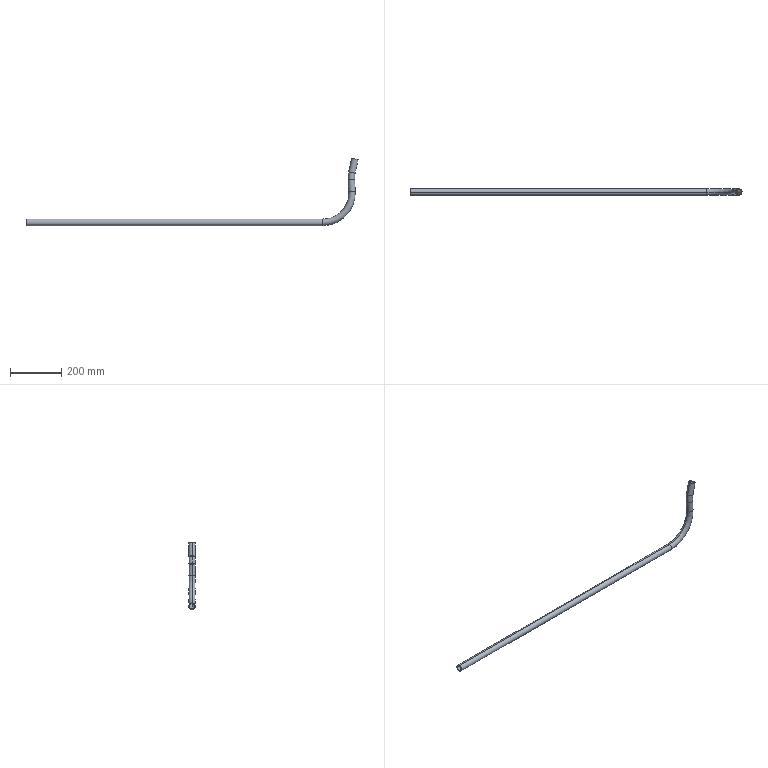Part | STEP file | PN_0018_Default<As Machined> | 1 solid | 26 faces | box 1294 x 25.4 x 262.259 mm | volume 292213 mm3 | cylinder 16 | torus 8 | plane 2 | commonest cylinder face diameters 19.8 x6 25.4 x6 4.2 x4
STEP:
#1=CARTESIAN_POINT('',(312.929,0.,218.744));
#2=VERTEX_POINT('',#1);
#3=CARTESIAN_POINT('',(293.156,0.,217.708));
#4=VERTEX_POINT('',#3);
#5=CARTESIAN_POINT('',(303.043,0.,218.226));
#6=DIRECTION('',(0.05234,0.,-0.9986));
#7=AXIS2_PLACEMENT_3D('',#5,#6,$);
#8=CIRCLE('',#7,9.9);
#9=EDGE_CURVE('',#2,#4,#8,.T.);
#10=ORIENTED_EDGE('',*,*,#9,.T.);
#11=CARTESIAN_POINT('',(295.612,0.,248.912));
#12=VERTEX_POINT('',#11);
#13=CARTESIAN_POINT('',(412.892,0.,223.983));
#14=DIRECTION('',(0.,1.,0.));
#15=AXIS2_PLACEMENT_3D('',#13,#14,$);
#16=CIRCLE('',#15,119.9);
#17=EDGE_CURVE('',#4,#12,#16,.T.);
#18=ORIENTED_EDGE('',*,*,#17,.T.);
#19=CARTESIAN_POINT('',(314.979,0.,244.795));
#20=VERTEX_POINT('',#19);
#21=CARTESIAN_POINT('',(305.296,0.,246.853));
#22=DIRECTION('',(-0.2079,0.,-0.9781));
#23=AXIS2_PLACEMENT_3D('',#21,#22,$);
#24=CIRCLE('',#23,9.9);
#25=EDGE_CURVE('',#20,#12,#24,.T.);
#26=ORIENTED_EDGE('',*,*,#25,.F.);
#27=CARTESIAN_POINT('',(412.892,0.,223.983));
#28=DIRECTION('',(0.,1.,0.));
#29=AXIS2_PLACEMENT_3D('',#27,#28,$);
#30=CIRCLE('',#29,100.1);
#31=EDGE_CURVE('',#2,#20,#30,.T.);
#32=ORIENTED_EDGE('',*,*,#31,.F.);
#33=EDGE_LOOP('',(#10,#18,#26,#32));
#34=FACE_OUTER_BOUND('',#33,.T.);
#35=CARTESIAN_POINT('',(412.892,0.,223.983));
#36=DIRECTION('',(0.,1.,0.));
#37=DIRECTION('',(0.,0.,-1.));
#38=AXIS2_PLACEMENT_3D('',#35,#36,#37);
#39=TOROIDAL_SURFACE('',#38,110.,9.9);
#40=ADVANCED_FACE('',(#34),#39,.F.);
#41=CARTESIAN_POINT('',(315.329,0.,172.946));
#42=VERTEX_POINT('',#41);
#43=CARTESIAN_POINT('',(295.556,0.,171.91));
#44=VERTEX_POINT('',#43);
#45=CARTESIAN_POINT('',(305.443,0.,172.428));
#46=DIRECTION('',(-0.05234,0.,0.9986));
#47=AXIS2_PLACEMENT_3D('',#45,#46,$);
#48=CIRCLE('',#47,9.9);
#49=EDGE_CURVE('',#42,#44,#48,.F.);
#50=ORIENTED_EDGE('',*,*,#49,.T.);
#51=CARTESIAN_POINT('',(295.556,0.,171.91));
#52=DIRECTION('',(-0.05234,0.,0.9986));
#53=VECTOR('',#52,1.);
#54=LINE('',#51,#53);
#55=EDGE_CURVE('',#44,#4,#54,.T.);
#56=ORIENTED_EDGE('',*,*,#55,.T.);
#57=ORIENTED_EDGE('',*,*,#9,.F.);
#58=CARTESIAN_POINT('',(315.329,0.,172.946));
#59=DIRECTION('',(-0.05234,0.,0.9986));
#60=VECTOR('',#59,1.);
#61=LINE('',#58,#60);
#62=EDGE_CURVE('',#42,#2,#61,.T.);
#63=ORIENTED_EDGE('',*,*,#62,.F.);
#64=EDGE_LOOP('',(#50,#56,#57,#63));
#65=FACE_OUTER_BOUND('',#64,.T.);
#66=CARTESIAN_POINT('',(305.443,0.,172.428));
#67=DIRECTION('',(-0.05234,0.,0.9986));
#68=DIRECTION('',(-0.9986,0.,-0.05234));
#69=AXIS2_PLACEMENT_3D('',#66,#67,#68);
#70=CYLINDRICAL_SURFACE('',#69,9.9);
#71=ADVANCED_FACE('',(#65),#70,.F.);
#72=ORIENTED_EDGE('',*,*,#17,.F.);
#73=CARTESIAN_POINT('',(303.043,0.,218.226));
#74=DIRECTION('',(0.05234,0.,-0.9986));
#75=AXIS2_PLACEMENT_3D('',#73,#74,$);
#76=CIRCLE('',#75,9.9);
#77=EDGE_CURVE('',#4,#2,#76,.T.);
#78=ORIENTED_EDGE('',*,*,#77,.T.);
#79=ORIENTED_EDGE('',*,*,#31,.T.);
#80=CARTESIAN_POINT('',(305.296,0.,246.853));
#81=DIRECTION('',(-0.2079,0.,-0.9781));
#82=AXIS2_PLACEMENT_3D('',#80,#81,$);
#83=CIRCLE('',#82,9.9);
#84=EDGE_CURVE('',#12,#20,#83,.T.);
#85=ORIENTED_EDGE('',*,*,#84,.F.);
#86=EDGE_LOOP('',(#72,#78,#79,#85));
#87=FACE_OUTER_BOUND('',#86,.T.);
#88=CARTESIAN_POINT('',(412.892,0.,223.983));
#89=DIRECTION('',(0.,1.,0.));
#90=DIRECTION('',(0.,0.,-1.));
#91=AXIS2_PLACEMENT_3D('',#88,#89,#90);
#92=TOROIDAL_SURFACE('',#91,110.,9.9);
#93=ADVANCED_FACE('',(#87),#92,.F.);
#94=ORIENTED_EDGE('',*,*,#25,.T.);
#95=CARTESIAN_POINT('',(306.777,0.,301.438));
#96=VERTEX_POINT('',#95);
#97=CARTESIAN_POINT('',(295.612,0.,248.912));
#98=DIRECTION('',(0.2079,0.,0.9781));
#99=VECTOR('',#98,1.);
#100=LINE('',#97,#99);
#101=EDGE_CURVE('',#12,#96,#100,.T.);
#102=ORIENTED_EDGE('',*,*,#101,.T.);
#103=CARTESIAN_POINT('',(326.144,0.,297.322));
#104=VERTEX_POINT('',#103);
#105=CARTESIAN_POINT('',(316.46,0.,299.38));
#106=DIRECTION('',(0.2079,0.,0.9781));
#107=AXIS2_PLACEMENT_3D('',#105,#106,$);
#108=CIRCLE('',#107,9.9);
#109=EDGE_CURVE('',#104,#96,#108,.F.);
#110=ORIENTED_EDGE('',*,*,#109,.F.);
#111=CARTESIAN_POINT('',(322.443,0.000000654,279.911));
#112=VERTEX_POINT('',#111);
#113=CARTESIAN_POINT('',(314.979,0.,244.795));
#114=DIRECTION('',(0.2079,0.,0.9781));
#115=VECTOR('',#114,1.);
#116=LINE('',#113,#115);
#117=EDGE_CURVE('',#112,#104,#116,.T.);
#118=ORIENTED_EDGE('',*,*,#117,.F.);
#119=CARTESIAN_POINT('',(321.57,0.000000654,275.802));
#120=VERTEX_POINT('',#119);
#121=CARTESIAN_POINT('',(321.57,0.,275.802));
#122=CARTESIAN_POINT('',(321.57,-0.1409,275.802));
#123=CARTESIAN_POINT('',(321.57,-0.2806,275.814));
#124=CARTESIAN_POINT('',(321.57,-0.4191,275.838));
#125=CARTESIAN_POINT('',(321.57,-0.6933,275.91));
#126=CARTESIAN_POINT('',(321.572,-0.9514,276.026));
#127=CARTESIAN_POINT('',(321.574,-1.075,276.096));
#128=CARTESIAN_POINT('',(321.583,-1.487,276.374));
#129=CARTESIAN_POINT('',(321.607,-1.81,276.764));
#130=CARTESIAN_POINT('',(321.64,-1.978,277.087));
#131=CARTESIAN_POINT('',(321.712,-2.113,277.567));
#132=CARTESIAN_POINT('',(321.817,-2.102,278.051));
#133=CARTESIAN_POINT('',(321.85,-2.086,278.189));
#134=CARTESIAN_POINT('',(321.936,-2.02,278.525));
#135=CARTESIAN_POINT('',(322.031,-1.883,278.838));
#136=CARTESIAN_POINT('',(322.09,-1.775,279.016));
#137=CARTESIAN_POINT('',(322.186,-1.56,279.285));
#138=CARTESIAN_POINT('',(322.271,-1.292,279.502));
#139=CARTESIAN_POINT('',(322.302,-1.177,279.58));
#140=CARTESIAN_POINT('',(322.369,-0.8901,279.743));
#141=CARTESIAN_POINT('',(322.416,-0.5741,279.849));
#142=CARTESIAN_POINT('',(322.434,-0.3859,279.889));
#143=CARTESIAN_POINT('',(322.443,-0.1923,279.911));
#144=CARTESIAN_POINT('',(322.443,0.,279.911));
#145=B_SPLINE_CURVE_WITH_KNOTS('',5,(#121,#122,#123,#124,#125,#126,#127,#128,#129,#130,#131,#132,#133,#134,#135,#136,#137,#138,#139,#140,#141,#142,#143,#144),.UNSPECIFIED.,.F.,.U.,(6,3,3,3,3,3,3,6),(0.,0.9925,1.996,4.5,5.493,6.994,8.001,9.365),.UNSPECIFIED.);
#146=EDGE_CURVE('',#120,#112,#145,.T.);
#147=ORIENTED_EDGE('',*,*,#146,.F.);
#148=CARTESIAN_POINT('',(314.979,0.,244.795));
#149=DIRECTION('',(0.2079,0.,0.9781));
#150=VECTOR('',#149,1.);
#151=LINE('',#148,#150);
#152=EDGE_CURVE('',#20,#120,#151,.T.);
#153=ORIENTED_EDGE('',*,*,#152,.F.);
#154=EDGE_LOOP('',(#94,#102,#110,#118,#147,#153));
#155=FACE_OUTER_BOUND('',#154,.T.);
#156=CARTESIAN_POINT('',(305.296,0.,246.853));
#157=DIRECTION('',(0.2079,0.,0.9781));
#158=DIRECTION('',(-0.9781,0.,0.2079));
#159=AXIS2_PLACEMENT_3D('',#156,#157,#158);
#160=CYLINDRICAL_SURFACE('',#159,9.9);
#161=ADVANCED_FACE('',(#155),#160,.F.);
#162=CARTESIAN_POINT('',(191.599,0.,42.562));
#163=VERTEX_POINT('',#162);
#164=CARTESIAN_POINT('',(191.599,0.,166.462));
#165=DIRECTION('',(0.,-1.,0.));
#166=AXIS2_PLACEMENT_3D('',#164,#165,$);
#167=CIRCLE('',#166,123.9);
#168=EDGE_CURVE('',#163,#42,#167,.T.);
#169=ORIENTED_EDGE('',*,*,#168,.F.);
#170=CARTESIAN_POINT('',(191.599,0.,62.362));
#171=VERTEX_POINT('',#170);
#172=CARTESIAN_POINT('',(191.599,0.,52.462));
#173=DIRECTION('',(-1.,0.,0.));
#174=AXIS2_PLACEMENT_3D('',#172,#173,$);
#175=CIRCLE('',#174,9.9);
#176=EDGE_CURVE('',#163,#171,#175,.T.);
#177=ORIENTED_EDGE('',*,*,#176,.T.);
#178=CARTESIAN_POINT('',(191.599,0.,166.462));
#179=DIRECTION('',(0.,-1.,0.));
#180=AXIS2_PLACEMENT_3D('',#178,#179,$);
#181=CIRCLE('',#180,104.1);
#182=EDGE_CURVE('',#171,#44,#181,.T.);
#183=ORIENTED_EDGE('',*,*,#182,.T.);
#184=ORIENTED_EDGE('',*,*,#49,.F.);
#185=EDGE_LOOP('',(#169,#177,#183,#184));
#186=FACE_OUTER_BOUND('',#185,.T.);
#187=CARTESIAN_POINT('',(191.599,0.,166.462));
#188=DIRECTION('',(0.,-1.,0.));
#189=DIRECTION('',(0.,0.,-1.));
#190=AXIS2_PLACEMENT_3D('',#187,#188,#189);
#191=TOROIDAL_SURFACE('',#190,114.,9.9);
#192=ADVANCED_FACE('',(#186),#191,.F.);
#193=ORIENTED_EDGE('',*,*,#55,.F.);
#194=CARTESIAN_POINT('',(305.443,0.,172.428));
#195=DIRECTION('',(-0.05234,0.,0.9986));
#196=AXIS2_PLACEMENT_3D('',#194,#195,$);
#197=CIRCLE('',#196,9.9);
#198=EDGE_CURVE('',#44,#42,#197,.F.);
#199=ORIENTED_EDGE('',*,*,#198,.T.);
#200=ORIENTED_EDGE('',*,*,#62,.T.);
#201=ORIENTED_EDGE('',*,*,#77,.F.);
#202=EDGE_LOOP('',(#193,#199,#200,#201));
#203=FACE_OUTER_BOUND('',#202,.T.);
#204=CARTESIAN_POINT('',(305.443,0.,172.428));
#205=DIRECTION('',(-0.05234,0.,0.9986));
#206=DIRECTION('',(0.9986,0.,0.05234));
#207=AXIS2_PLACEMENT_3D('',#204,#205,#206);
#208=CYLINDRICAL_SURFACE('',#207,9.9);
#209=ADVANCED_FACE('',(#203),#208,.F.);
#210=ORIENTED_EDGE('',*,*,#101,.F.);
#211=ORIENTED_EDGE('',*,*,#84,.T.);
#212=ORIENTED_EDGE('',*,*,#152,.T.);
#213=CARTESIAN_POINT('',(322.443,0.,279.911));
#214=CARTESIAN_POINT('',(322.443,0.3529,279.91));
#215=CARTESIAN_POINT('',(322.412,0.7056,279.841));
#216=CARTESIAN_POINT('',(322.35,1.039,279.702));
#217=CARTESIAN_POINT('',(322.235,1.443,279.423));
#218=CARTESIAN_POINT('',(322.103,1.742,279.048));
#219=CARTESIAN_POINT('',(322.064,1.818,278.934));
#220=CARTESIAN_POINT('',(321.969,1.98,278.637));
#221=CARTESIAN_POINT('',(321.878,2.074,278.307));
#222=CARTESIAN_POINT('',(321.827,2.106,278.101));
#223=CARTESIAN_POINT('',(321.707,2.118,277.546));
#224=CARTESIAN_POINT('',(321.63,1.94,277.003));
#225=CARTESIAN_POINT('',(321.601,1.758,276.686));
#226=CARTESIAN_POINT('',(321.574,1.336,276.218));
#227=CARTESIAN_POINT('',(321.57,0.7828,275.93));
#228=CARTESIAN_POINT('',(321.57,0.528,275.845));
#229=CARTESIAN_POINT('',(321.57,0.2647,275.802));
#230=CARTESIAN_POINT('',(321.57,0.000000654,275.802));
#231=B_SPLINE_CURVE_WITH_KNOTS('',5,(#213,#214,#215,#216,#217,#218,#219,#220,#221,#222,#223,#224,#225,#226,#227,#228,#229,#230),.UNSPECIFIED.,.F.,.U.,(6,3,3,3,3,6),(0.,2.501,3.504,4.993,7.498,9.366),.UNSPECIFIED.);
#232=EDGE_CURVE('',#112,#120,#231,.T.);
#233=ORIENTED_EDGE('',*,*,#232,.F.);
#234=ORIENTED_EDGE('',*,*,#117,.T.);
#235=CARTESIAN_POINT('',(316.46,0.,299.38));
#236=DIRECTION('',(0.2079,0.,0.9781));
#237=AXIS2_PLACEMENT_3D('',#235,#236,$);
#238=CIRCLE('',#237,9.9);
#239=EDGE_CURVE('',#96,#104,#238,.F.);
#240=ORIENTED_EDGE('',*,*,#239,.F.);
#241=EDGE_LOOP('',(#210,#211,#212,#233,#234,#240));
#242=FACE_OUTER_BOUND('',#241,.T.);
#243=CARTESIAN_POINT('',(305.296,0.,246.853));
#244=DIRECTION('',(0.2079,0.,0.9781));
#245=DIRECTION('',(0.9781,0.,-0.2079));
#246=AXIS2_PLACEMENT_3D('',#243,#244,#245);
#247=CYLINDRICAL_SURFACE('',#246,9.9);
#248=ADVANCED_FACE('',(#242),#247,.F.);
#249=CARTESIAN_POINT('',(328.883,0.,296.739));
#250=VERTEX_POINT('',#249);
#251=CARTESIAN_POINT('',(304.038,0.,302.02));
#252=VERTEX_POINT('',#251);
#253=CARTESIAN_POINT('',(316.46,0.,299.38));
#254=DIRECTION('',(0.2079,0.,0.9781));
#255=AXIS2_PLACEMENT_3D('',#253,#254,$);
#256=CIRCLE('',#255,12.7);
#257=EDGE_CURVE('',#250,#252,#256,.T.);
#258=ORIENTED_EDGE('',*,*,#257,.T.);
#259=CARTESIAN_POINT('',(316.46,0.,299.38));
#260=DIRECTION('',(0.2079,0.,0.9781));
#261=AXIS2_PLACEMENT_3D('',#259,#260,$);
#262=CIRCLE('',#261,12.7);
#263=EDGE_CURVE('',#252,#250,#262,.T.);
#264=ORIENTED_EDGE('',*,*,#263,.T.);
#265=EDGE_LOOP('',(#258,#264));
#266=FACE_OUTER_BOUND('',#265,.T.);
#267=ORIENTED_EDGE('',*,*,#109,.T.);
#268=ORIENTED_EDGE('',*,*,#239,.T.);
#269=EDGE_LOOP('',(#267,#268));
#270=FACE_BOUND('',#269,.T.);
#271=CARTESIAN_POINT('',(316.46,0.,299.38));
#272=DIRECTION('',(0.2079,0.,0.9781));
#273=DIRECTION('',(0.9781,0.,-0.2079));
#274=AXIS2_PLACEMENT_3D('',#271,#272,#273);
#275=PLANE('',#274);
#276=ADVANCED_FACE('',(#266,#270),#275,.T.);
#277=ORIENTED_EDGE('',*,*,#146,.T.);
#278=CARTESIAN_POINT('',(325.182,0.,279.328));
#279=VERTEX_POINT('',#278);
#280=CARTESIAN_POINT('',(-914.113,-0.00004482,542.749));
#281=DIRECTION('',(0.9781,0.000000036,-0.2079));
#282=VECTOR('',#281,1.);
#283=LINE('',#280,#282);
#284=EDGE_CURVE('',#112,#279,#283,.T.);
#285=ORIENTED_EDGE('',*,*,#284,.T.);
#286=CARTESIAN_POINT('',(324.309,0.000000755,275.22));
#287=VERTEX_POINT('',#286);
#288=CARTESIAN_POINT('',(325.182,0.,279.328));
#289=CARTESIAN_POINT('',(325.182,-0.2107,279.328));
#290=CARTESIAN_POINT('',(325.172,-0.4213,279.304));
#291=CARTESIAN_POINT('',(325.152,-0.6318,279.252));
#292=CARTESIAN_POINT('',(325.105,-0.962,279.128));
#293=CARTESIAN_POINT('',(325.037,-1.256,278.942));
#294=CARTESIAN_POINT('',(325.007,-1.368,278.857));
#295=CARTESIAN_POINT('',(324.942,-1.577,278.669));
#296=CARTESIAN_POINT('',(324.872,-1.75,278.449));
#297=CARTESIAN_POINT('',(324.84,-1.818,278.345));
#298=CARTESIAN_POINT('',(324.75,-1.982,278.041));
#299=CARTESIAN_POINT('',(324.662,-2.077,277.705));
#300=CARTESIAN_POINT('',(324.613,-2.107,277.499));
#301=CARTESIAN_POINT('',(324.539,-2.113,277.153));
#302=CARTESIAN_POINT('',(324.478,-2.045,276.812));
#303=CARTESIAN_POINT('',(324.455,-2.005,276.675));
#304=CARTESIAN_POINT('',(324.415,-1.904,276.409));
#305=CARTESIAN_POINT('',(324.385,-1.758,276.163));
#306=CARTESIAN_POINT('',(324.373,-1.685,276.06));
#307=CARTESIAN_POINT('',(324.348,-1.484,275.818));
#308=CARTESIAN_POINT('',(324.332,-1.241,275.618));
#309=CARTESIAN_POINT('',(324.326,-1.103,275.525));
#310=CARTESIAN_POINT('',(324.316,-0.8143,275.369));
#311=CARTESIAN_POINT('',(324.311,-0.5004,275.271));
#312=CARTESIAN_POINT('',(324.309,-0.3375,275.237));
#313=CARTESIAN_POINT('',(324.309,-0.169,275.22));
#314=CARTESIAN_POINT('',(324.309,0.000000457,275.22));
#315=B_SPLINE_CURVE_WITH_KNOTS('',5,(#288,#289,#290,#291,#292,#293,#294,#295,#296,#297,#298,#299,#300,#301,#302,#303,#304,#305,#306,#307,#308,#309,#310,#311,#312,#313,#314),.UNSPECIFIED.,.F.,.U.,(6,3,3,3,3,3,3,3,6),(0.,1.493,2.499,3.529,5.024,6.022,7.055,8.245,9.436),.UNSPECIFIED.);
#316=EDGE_CURVE('',#279,#287,#315,.T.);
#317=ORIENTED_EDGE('',*,*,#316,.T.);
#318=CARTESIAN_POINT('',(-914.986,-0.00004482,538.641));
#319=DIRECTION('',(0.9781,0.000000036,-0.2079));
#320=VECTOR('',#319,1.);
#321=LINE('',#318,#320);
#322=EDGE_CURVE('',#120,#287,#321,.T.);
#323=ORIENTED_EDGE('',*,*,#322,.F.);
#324=EDGE_LOOP('',(#277,#285,#317,#323));
#325=FACE_OUTER_BOUND('',#324,.T.);
#326=CARTESIAN_POINT('',(-914.55,-0.00004482,540.695));
#327=DIRECTION('',(0.9781,0.000000036,-0.2079));
#328=DIRECTION('',(0.2079,0.,0.9781));
#329=AXIS2_PLACEMENT_3D('',#326,#327,#328);
#330=CYLINDRICAL_SURFACE('',#329,2.1);
#331=ADVANCED_FACE('',(#325),#330,.F.);
#332=CARTESIAN_POINT('',(191.599,0.,52.462));
#333=DIRECTION('',(-1.,0.,0.));
#334=AXIS2_PLACEMENT_3D('',#332,#333,$);
#335=CIRCLE('',#334,9.9);
#336=EDGE_CURVE('',#171,#163,#335,.T.);
#337=ORIENTED_EDGE('',*,*,#336,.T.);
#338=ORIENTED_EDGE('',*,*,#168,.T.);
#339=ORIENTED_EDGE('',*,*,#198,.F.);
#340=ORIENTED_EDGE('',*,*,#182,.F.);
#341=EDGE_LOOP('',(#337,#338,#339,#340));
#342=FACE_OUTER_BOUND('',#341,.T.);
#343=CARTESIAN_POINT('',(191.599,0.,166.462));
#344=DIRECTION('',(0.,-1.,0.));
#345=DIRECTION('',(0.,0.,-1.));
#346=AXIS2_PLACEMENT_3D('',#343,#344,#345);
#347=TOROIDAL_SURFACE('',#346,114.,9.9);
#348=ADVANCED_FACE('',(#342),#347,.F.);
#349=CARTESIAN_POINT('',(-965.28,0.,42.562));
#350=VERTEX_POINT('',#349);
#351=CARTESIAN_POINT('',(-965.28,0.,62.362));
#352=VERTEX_POINT('',#351);
#353=CARTESIAN_POINT('',(-965.28,0.,52.462));
#354=DIRECTION('',(1.,0.,0.));
#355=AXIS2_PLACEMENT_3D('',#353,#354,$);
#356=CIRCLE('',#355,9.9);
#357=EDGE_CURVE('',#350,#352,#356,.F.);
#358=ORIENTED_EDGE('',*,*,#357,.T.);
#359=CARTESIAN_POINT('',(-965.28,0.,62.362));
#360=DIRECTION('',(1.,0.,0.));
#361=VECTOR('',#360,1.);
#362=LINE('',#359,#361);
#363=EDGE_CURVE('',#352,#171,#362,.T.);
#364=ORIENTED_EDGE('',*,*,#363,.T.);
#365=ORIENTED_EDGE('',*,*,#176,.F.);
#366=CARTESIAN_POINT('',(-948.18,0.,42.562));
#367=VERTEX_POINT('',#366);
#368=CARTESIAN_POINT('',(-965.28,0.,42.562));
#369=DIRECTION('',(1.,0.,0.));
#370=VECTOR('',#369,1.);
#371=LINE('',#368,#370);
#372=EDGE_CURVE('',#367,#163,#371,.T.);
#373=ORIENTED_EDGE('',*,*,#372,.F.);
#374=CARTESIAN_POINT('',(-952.38,0.,42.562));
#375=VERTEX_POINT('',#374);
#376=CARTESIAN_POINT('',(-952.38,0.,42.562));
#377=CARTESIAN_POINT('',(-952.38,-0.1409,42.562));
#378=CARTESIAN_POINT('',(-952.369,-0.2806,42.564));
#379=CARTESIAN_POINT('',(-952.345,-0.4191,42.569));
#380=CARTESIAN_POINT('',(-952.275,-0.6933,42.584));
#381=CARTESIAN_POINT('',(-952.161,-0.9514,42.606));
#382=CARTESIAN_POINT('',(-952.092,-1.075,42.619));
#383=CARTESIAN_POINT('',(-951.818,-1.487,42.668));
#384=CARTESIAN_POINT('',(-951.431,-1.81,42.725));
#385=CARTESIAN_POINT('',(-951.109,-1.978,42.76));
#386=CARTESIAN_POINT('',(-950.625,-2.113,42.789));
#387=CARTESIAN_POINT('',(-950.13,-2.102,42.787));
#388=CARTESIAN_POINT('',(-949.987,-2.086,42.784));
#389=CARTESIAN_POINT('',(-949.64,-2.02,42.77));
#390=CARTESIAN_POINT('',(-949.315,-1.883,42.742));
#391=CARTESIAN_POINT('',(-949.129,-1.775,42.721));
#392=CARTESIAN_POINT('',(-948.846,-1.56,42.683));
#393=CARTESIAN_POINT('',(-948.616,-1.292,42.645));
#394=CARTESIAN_POINT('',(-948.533,-1.177,42.631));
#395=CARTESIAN_POINT('',(-948.36,-0.8901,42.599));
#396=CARTESIAN_POINT('',(-948.246,-0.5741,42.576));
#397=CARTESIAN_POINT('',(-948.203,-0.3859,42.566));
#398=CARTESIAN_POINT('',(-948.18,-0.1923,42.562));
#399=CARTESIAN_POINT('',(-948.18,0.,42.562));
#400=B_SPLINE_CURVE_WITH_KNOTS('',5,(#376,#377,#378,#379,#380,#381,#382,#383,#384,#385,#386,#387,#388,#389,#390,#391,#392,#393,#394,#395,#396,#397,#398,#399),.UNSPECIFIED.,.F.,.U.,(6,3,3,3,3,3,3,6),(0.,0.9925,1.996,4.5,5.493,6.994,8.001,9.365),.UNSPECIFIED.);
#401=EDGE_CURVE('',#375,#367,#400,.T.);
#402=ORIENTED_EDGE('',*,*,#401,.F.);
#403=CARTESIAN_POINT('',(-965.28,0.,42.562));
#404=DIRECTION('',(1.,0.,0.));
#405=VECTOR('',#404,1.);
#406=LINE('',#403,#405);
#407=EDGE_CURVE('',#350,#375,#406,.T.);
#408=ORIENTED_EDGE('',*,*,#407,.F.);
#409=EDGE_LOOP('',(#358,#364,#365,#373,#402,#408));
#410=FACE_OUTER_BOUND('',#409,.T.);
#411=CARTESIAN_POINT('',(-965.28,0.,52.462));
#412=DIRECTION('',(1.,0.,0.));
#413=DIRECTION('',(0.,0.,1.));
#414=AXIS2_PLACEMENT_3D('',#411,#412,#413);
#415=CYLINDRICAL_SURFACE('',#414,9.9);
#416=ADVANCED_FACE('',(#410),#415,.F.);
#417=ORIENTED_EDGE('',*,*,#284,.F.);
#418=ORIENTED_EDGE('',*,*,#232,.T.);
#419=ORIENTED_EDGE('',*,*,#322,.T.);
#420=CARTESIAN_POINT('',(324.309,0.000000755,275.22));
#421=CARTESIAN_POINT('',(324.309,0.1416,275.22));
#422=CARTESIAN_POINT('',(324.309,0.2819,275.232));
#423=CARTESIAN_POINT('',(324.31,0.4206,275.256));
#424=CARTESIAN_POINT('',(324.314,0.695,275.327));
#425=CARTESIAN_POINT('',(324.321,0.9531,275.443));
#426=CARTESIAN_POINT('',(324.325,1.08,275.514));
#427=CARTESIAN_POINT('',(324.339,1.371,275.71));
#428=CARTESIAN_POINT('',(324.362,1.618,275.962));
#429=CARTESIAN_POINT('',(324.381,1.755,276.144));
#430=CARTESIAN_POINT('',(324.427,1.964,276.509));
#431=CARTESIAN_POINT('',(324.494,2.076,276.91));
#432=CARTESIAN_POINT('',(324.533,2.107,277.123));
#433=CARTESIAN_POINT('',(324.65,2.116,277.68));
#434=CARTESIAN_POINT('',(324.793,1.936,278.208));
#435=CARTESIAN_POINT('',(324.887,1.752,278.509));
#436=CARTESIAN_POINT('',(325.007,1.412,278.863));
#437=CARTESIAN_POINT('',(325.096,0.9854,279.104));
#438=CARTESIAN_POINT('',(325.118,0.8618,279.161));
#439=CARTESIAN_POINT('',(325.152,0.6171,279.251));
#440=CARTESIAN_POINT('',(325.172,0.3602,279.304));
#441=CARTESIAN_POINT('',(325.179,0.2405,279.32));
#442=CARTESIAN_POINT('',(325.182,0.12,279.328));
#443=CARTESIAN_POINT('',(325.182,0.000000755,279.328));
#444=B_SPLINE_CURVE_WITH_KNOTS('',5,(#420,#421,#422,#423,#424,#425,#426,#427,#428,#429,#430,#431,#432,#433,#434,#435,#436,#437,#438,#439,#440,#441,#442,#443),.UNSPECIFIED.,.F.,.U.,(6,3,3,3,3,3,3,6),(0.,0.997,1.996,3.478,4.966,7.469,8.479,9.33),.UNSPECIFIED.);
#445=EDGE_CURVE('',#287,#279,#444,.T.);
#446=ORIENTED_EDGE('',*,*,#445,.T.);
#447=EDGE_LOOP('',(#417,#418,#419,#446));
#448=FACE_OUTER_BOUND('',#447,.T.);
#449=CARTESIAN_POINT('',(-914.55,-0.00004482,540.695));
#450=DIRECTION('',(0.9781,0.000000036,-0.2079));
#451=DIRECTION('',(-0.2079,0.,-0.9781));
#452=AXIS2_PLACEMENT_3D('',#449,#450,#451);
#453=CYLINDRICAL_SURFACE('',#452,2.1);
#454=ADVANCED_FACE('',(#448),#453,.F.);
#455=CARTESIAN_POINT('',(317.718,0.,244.213));
#456=VERTEX_POINT('',#455);
#457=CARTESIAN_POINT('',(292.873,0.,249.494));
#458=VERTEX_POINT('',#457);
#459=CARTESIAN_POINT('',(305.296,0.,246.853));
#460=DIRECTION('',(0.2079,0.,0.9781));
#461=AXIS2_PLACEMENT_3D('',#459,#460,$);
#462=CIRCLE('',#461,12.7);
#463=EDGE_CURVE('',#456,#458,#462,.T.);
#464=ORIENTED_EDGE('',*,*,#463,.T.);
#465=CARTESIAN_POINT('',(292.873,0.,249.494));
#466=DIRECTION('',(0.2079,0.,0.9781));
#467=VECTOR('',#466,1.);
#468=LINE('',#465,#467);
#469=EDGE_CURVE('',#458,#252,#468,.T.);
#470=ORIENTED_EDGE('',*,*,#469,.T.);
#471=ORIENTED_EDGE('',*,*,#257,.F.);
#472=CARTESIAN_POINT('',(317.718,0.,244.213));
#473=DIRECTION('',(0.2079,0.,0.9781));
#474=VECTOR('',#473,1.);
#475=LINE('',#472,#474);
#476=EDGE_CURVE('',#279,#250,#475,.T.);
#477=ORIENTED_EDGE('',*,*,#476,.F.);
#478=ORIENTED_EDGE('',*,*,#445,.F.);
#479=CARTESIAN_POINT('',(317.718,0.,244.213));
#480=DIRECTION('',(0.2079,0.,0.9781));
#481=VECTOR('',#480,1.);
#482=LINE('',#479,#481);
#483=EDGE_CURVE('',#456,#287,#482,.T.);
#484=ORIENTED_EDGE('',*,*,#483,.F.);
#485=EDGE_LOOP('',(#464,#470,#471,#477,#478,#484));
#486=FACE_OUTER_BOUND('',#485,.T.);
#487=CARTESIAN_POINT('',(305.296,0.,246.853));
#488=DIRECTION('',(0.2079,0.,0.9781));
#489=DIRECTION('',(0.9781,0.,-0.2079));
#490=AXIS2_PLACEMENT_3D('',#487,#488,#489);
#491=CYLINDRICAL_SURFACE('',#490,12.7);
#492=ADVANCED_FACE('',(#486),#491,.T.);
#493=ORIENTED_EDGE('',*,*,#469,.F.);
#494=CARTESIAN_POINT('',(305.296,0.,246.853));
#495=DIRECTION('',(0.2079,0.,0.9781));
#496=AXIS2_PLACEMENT_3D('',#494,#495,$);
#497=CIRCLE('',#496,12.7);
#498=EDGE_CURVE('',#458,#456,#497,.T.);
#499=ORIENTED_EDGE('',*,*,#498,.T.);
#500=ORIENTED_EDGE('',*,*,#483,.T.);
#501=ORIENTED_EDGE('',*,*,#316,.F.);
#502=ORIENTED_EDGE('',*,*,#476,.T.);
#503=ORIENTED_EDGE('',*,*,#263,.F.);
#504=EDGE_LOOP('',(#493,#499,#500,#501,#502,#503));
#505=FACE_OUTER_BOUND('',#504,.T.);
#506=CARTESIAN_POINT('',(305.296,0.,246.853));
#507=DIRECTION('',(0.2079,0.,0.9781));
#508=DIRECTION('',(-0.9781,0.,0.2079));
#509=AXIS2_PLACEMENT_3D('',#506,#507,#508);
#510=CYLINDRICAL_SURFACE('',#509,12.7);
#511=ADVANCED_FACE('',(#505),#510,.T.);
#512=ORIENTED_EDGE('',*,*,#363,.F.);
#513=CARTESIAN_POINT('',(-965.28,0.,52.462));
#514=DIRECTION('',(1.,0.,0.));
#515=AXIS2_PLACEMENT_3D('',#513,#514,$);
#516=CIRCLE('',#515,9.9);
#517=EDGE_CURVE('',#352,#350,#516,.F.);
#518=ORIENTED_EDGE('',*,*,#517,.T.);
#519=ORIENTED_EDGE('',*,*,#407,.T.);
#520=CARTESIAN_POINT('',(-948.18,0.,42.562));
#521=CARTESIAN_POINT('',(-948.181,0.3529,42.562));
#522=CARTESIAN_POINT('',(-948.255,0.7056,42.577));
#523=CARTESIAN_POINT('',(-948.403,1.039,42.609));
#524=CARTESIAN_POINT('',(-948.7,1.443,42.664));
#525=CARTESIAN_POINT('',(-949.095,1.742,42.715));
#526=CARTESIAN_POINT('',(-949.214,1.818,42.729));
#527=CARTESIAN_POINT('',(-949.525,1.98,42.761));
#528=CARTESIAN_POINT('',(-949.866,2.074,42.781));
#529=CARTESIAN_POINT('',(-950.079,2.106,42.788));
#530=CARTESIAN_POINT('',(-950.646,2.118,42.791));
#531=CARTESIAN_POINT('',(-951.194,1.94,42.753));
#532=CARTESIAN_POINT('',(-951.509,1.758,42.715));
#533=CARTESIAN_POINT('',(-951.973,1.336,42.644));
#534=CARTESIAN_POINT('',(-952.255,0.7828,42.588));
#535=CARTESIAN_POINT('',(-952.339,0.528,42.57));
#536=CARTESIAN_POINT('',(-952.38,0.2647,42.562));
#537=CARTESIAN_POINT('',(-952.38,0.,42.562));
#538=B_SPLINE_CURVE_WITH_KNOTS('',5,(#520,#521,#522,#523,#524,#525,#526,#527,#528,#529,#530,#531,#532,#533,#534,#535,#536,#537),.UNSPECIFIED.,.F.,.U.,(6,3,3,3,3,6),(0.,2.501,3.504,4.993,7.498,9.366),.UNSPECIFIED.);
#539=EDGE_CURVE('',#367,#375,#538,.T.);
#540=ORIENTED_EDGE('',*,*,#539,.F.);
#541=ORIENTED_EDGE('',*,*,#372,.T.);
#542=ORIENTED_EDGE('',*,*,#336,.F.);
#543=EDGE_LOOP('',(#512,#518,#519,#540,#541,#542));
#544=FACE_OUTER_BOUND('',#543,.T.);
#545=CARTESIAN_POINT('',(-965.28,0.,52.462));
#546=DIRECTION('',(1.,0.,0.));
#547=DIRECTION('',(0.,0.,-1.));
#548=AXIS2_PLACEMENT_3D('',#545,#546,#547);
#549=CYLINDRICAL_SURFACE('',#548,9.9);
#550=ADVANCED_FACE('',(#544),#549,.F.);
#551=CARTESIAN_POINT('',(-965.28,0.,39.762));
#552=VERTEX_POINT('',#551);
#553=CARTESIAN_POINT('',(-965.28,0.,65.162));
#554=VERTEX_POINT('',#553);
#555=CARTESIAN_POINT('',(-965.28,0.,52.462));
#556=DIRECTION('',(1.,0.,0.));
#557=AXIS2_PLACEMENT_3D('',#555,#556,$);
#558=CIRCLE('',#557,12.7);
#559=EDGE_CURVE('',#552,#554,#558,.T.);
#560=ORIENTED_EDGE('',*,*,#559,.F.);
#561=CARTESIAN_POINT('',(-965.28,0.,52.462));
#562=DIRECTION('',(1.,0.,0.));
#563=AXIS2_PLACEMENT_3D('',#561,#562,$);
#564=CIRCLE('',#563,12.7);
#565=EDGE_CURVE('',#554,#552,#564,.T.);
#566=ORIENTED_EDGE('',*,*,#565,.F.);
#567=EDGE_LOOP('',(#560,#566));
#568=FACE_OUTER_BOUND('',#567,.T.);
#569=ORIENTED_EDGE('',*,*,#357,.F.);
#570=ORIENTED_EDGE('',*,*,#517,.F.);
#571=EDGE_LOOP('',(#569,#570));
#572=FACE_BOUND('',#571,.T.);
#573=CARTESIAN_POINT('',(-965.28,0.,52.462));
#574=DIRECTION('',(1.,0.,0.));
#575=DIRECTION('',(0.,0.,-1.));
#576=AXIS2_PLACEMENT_3D('',#573,#574,#575);
#577=PLANE('',#576);
#578=ADVANCED_FACE('',(#568,#572),#577,.F.);
#579=ORIENTED_EDGE('',*,*,#401,.T.);
#580=CARTESIAN_POINT('',(-948.18,0.,39.762));
#581=VERTEX_POINT('',#580);
#582=CARTESIAN_POINT('',(-948.18,0.,302.021));
#583=DIRECTION('',(0.,0.,-1.));
#584=VECTOR('',#583,1.);
#585=LINE('',#582,#584);
#586=EDGE_CURVE('',#367,#581,#585,.T.);
#587=ORIENTED_EDGE('',*,*,#586,.T.);
#588=CARTESIAN_POINT('',(-952.38,0.,39.762));
#589=VERTEX_POINT('',#588);
#590=CARTESIAN_POINT('',(-948.18,0.,39.762));
#591=CARTESIAN_POINT('',(-948.18,-0.2107,39.762));
#592=CARTESIAN_POINT('',(-948.207,-0.4213,39.766));
#593=CARTESIAN_POINT('',(-948.261,-0.6318,39.775));
#594=CARTESIAN_POINT('',(-948.392,-0.962,39.796));
#595=CARTESIAN_POINT('',(-948.588,-1.256,39.823));
#596=CARTESIAN_POINT('',(-948.677,-1.368,39.835));
#597=CARTESIAN_POINT('',(-948.875,-1.577,39.859));
#598=CARTESIAN_POINT('',(-949.105,-1.75,39.882));
#599=CARTESIAN_POINT('',(-949.213,-1.818,39.892));
#600=CARTESIAN_POINT('',(-949.529,-1.982,39.917));
#601=CARTESIAN_POINT('',(-949.876,-2.077,39.932));
#602=CARTESIAN_POINT('',(-950.088,-2.107,39.938));
#603=CARTESIAN_POINT('',(-950.442,-2.113,39.938));
#604=CARTESIAN_POINT('',(-950.788,-2.045,39.927));
#605=CARTESIAN_POINT('',(-950.927,-2.005,39.921));
#606=CARTESIAN_POINT('',(-951.195,-1.904,39.905));
#607=CARTESIAN_POINT('',(-951.442,-1.758,39.883));
#608=CARTESIAN_POINT('',(-951.546,-1.685,39.873));
#609=CARTESIAN_POINT('',(-951.787,-1.484,39.847));
#610=CARTESIAN_POINT('',(-951.987,-1.241,39.821));
#611=CARTESIAN_POINT('',(-952.078,-1.103,39.808));
#612=CARTESIAN_POINT('',(-952.233,-0.8143,39.785));
#613=CARTESIAN_POINT('',(-952.33,-0.5004,39.77));
#614=CARTESIAN_POINT('',(-952.363,-0.3375,39.764));
#615=CARTESIAN_POINT('',(-952.38,-0.169,39.762));
#616=CARTESIAN_POINT('',(-952.38,0.,39.762));
#617=B_SPLINE_CURVE_WITH_KNOTS('',5,(#590,#591,#592,#593,#594,#595,#596,#597,#598,#599,#600,#601,#602,#603,#604,#605,#606,#607,#608,#609,#610,#611,#612,#613,#614,#615,#616),.UNSPECIFIED.,.F.,.U.,(6,3,3,3,3,3,3,3,6),(0.,1.493,2.499,3.529,5.024,6.022,7.055,8.245,9.436),.UNSPECIFIED.);
#618=EDGE_CURVE('',#581,#589,#617,.T.);
#619=ORIENTED_EDGE('',*,*,#618,.T.);
#620=CARTESIAN_POINT('',(-952.38,0.,302.021));
#621=DIRECTION('',(0.,0.,-1.));
#622=VECTOR('',#621,1.);
#623=LINE('',#620,#622);
#624=EDGE_CURVE('',#375,#589,#623,.T.);
#625=ORIENTED_EDGE('',*,*,#624,.F.);
#626=EDGE_LOOP('',(#579,#587,#619,#625));
#627=FACE_OUTER_BOUND('',#626,.T.);
#628=CARTESIAN_POINT('',(-950.28,0.,302.021));
#629=DIRECTION('',(0.,0.,-1.));
#630=DIRECTION('',(1.,0.,0.));
#631=AXIS2_PLACEMENT_3D('',#628,#629,#630);
#632=CYLINDRICAL_SURFACE('',#631,2.1);
#633=ADVANCED_FACE('',(#627),#632,.F.);
#634=CARTESIAN_POINT('',(315.725,0.,218.891));
#635=VERTEX_POINT('',#634);
#636=CARTESIAN_POINT('',(290.36,0.,217.561));
#637=VERTEX_POINT('',#636);
#638=CARTESIAN_POINT('',(303.043,0.,218.226));
#639=DIRECTION('',(0.05234,0.,-0.9986));
#640=AXIS2_PLACEMENT_3D('',#638,#639,$);
#641=CIRCLE('',#640,12.7);
#642=EDGE_CURVE('',#635,#637,#641,.F.);
#643=ORIENTED_EDGE('',*,*,#642,.T.);
#644=CARTESIAN_POINT('',(412.892,0.,223.983));
#645=DIRECTION('',(0.,1.,0.));
#646=AXIS2_PLACEMENT_3D('',#644,#645,$);
#647=CIRCLE('',#646,122.7);
#648=EDGE_CURVE('',#637,#458,#647,.T.);
#649=ORIENTED_EDGE('',*,*,#648,.T.);
#650=ORIENTED_EDGE('',*,*,#463,.F.);
#651=CARTESIAN_POINT('',(412.892,0.,223.983));
#652=DIRECTION('',(0.,1.,0.));
#653=AXIS2_PLACEMENT_3D('',#651,#652,$);
#654=CIRCLE('',#653,97.3);
#655=EDGE_CURVE('',#635,#456,#654,.T.);
#656=ORIENTED_EDGE('',*,*,#655,.F.);
#657=EDGE_LOOP('',(#643,#649,#650,#656));
#658=FACE_OUTER_BOUND('',#657,.T.);
#659=CARTESIAN_POINT('',(412.892,0.,223.983));
#660=DIRECTION('',(0.,1.,0.));
#661=DIRECTION('',(0.,0.,-1.));
#662=AXIS2_PLACEMENT_3D('',#659,#660,#661);
#663=TOROIDAL_SURFACE('',#662,110.,12.7);
#664=ADVANCED_FACE('',(#658),#663,.T.);
#665=ORIENTED_EDGE('',*,*,#648,.F.);
#666=CARTESIAN_POINT('',(303.043,0.,218.226));
#667=DIRECTION('',(0.05234,0.,-0.9986));
#668=AXIS2_PLACEMENT_3D('',#666,#667,$);
#669=CIRCLE('',#668,12.7);
#670=EDGE_CURVE('',#637,#635,#669,.F.);
#671=ORIENTED_EDGE('',*,*,#670,.T.);
#672=ORIENTED_EDGE('',*,*,#655,.T.);
#673=ORIENTED_EDGE('',*,*,#498,.F.);
#674=EDGE_LOOP('',(#665,#671,#672,#673));
#675=FACE_OUTER_BOUND('',#674,.T.);
#676=CARTESIAN_POINT('',(412.892,0.,223.983));
#677=DIRECTION('',(0.,1.,0.));
#678=DIRECTION('',(0.,0.,-1.));
#679=AXIS2_PLACEMENT_3D('',#676,#677,#678);
#680=TOROIDAL_SURFACE('',#679,110.,12.7);
#681=ADVANCED_FACE('',(#675),#680,.T.);
#682=ORIENTED_EDGE('',*,*,#586,.F.);
#683=ORIENTED_EDGE('',*,*,#539,.T.);
#684=ORIENTED_EDGE('',*,*,#624,.T.);
#685=CARTESIAN_POINT('',(-952.38,0.,39.762));
#686=CARTESIAN_POINT('',(-952.38,0.1416,39.762));
#687=CARTESIAN_POINT('',(-952.368,0.2819,39.763));
#688=CARTESIAN_POINT('',(-952.345,0.4206,39.767));
#689=CARTESIAN_POINT('',(-952.274,0.695,39.779));
#690=CARTESIAN_POINT('',(-952.159,0.9531,39.796));
#691=CARTESIAN_POINT('',(-952.09,1.08,39.807));
#692=CARTESIAN_POINT('',(-951.895,1.371,39.834));
#693=CARTESIAN_POINT('',(-951.643,1.618,39.864));
#694=CARTESIAN_POINT('',(-951.461,1.755,39.883));
#695=CARTESIAN_POINT('',(-951.095,1.964,39.914));
#696=CARTESIAN_POINT('',(-950.689,2.076,39.932));
#697=CARTESIAN_POINT('',(-950.473,2.107,39.938));
#698=CARTESIAN_POINT('',(-949.903,2.116,39.939));
#699=CARTESIAN_POINT('',(-949.357,1.936,39.909));
#700=CARTESIAN_POINT('',(-949.043,1.752,39.88));
#701=CARTESIAN_POINT('',(-948.672,1.412,39.836));
#702=CARTESIAN_POINT('',(-948.417,0.9854,39.799));
#703=CARTESIAN_POINT('',(-948.357,0.8618,39.79));
#704=CARTESIAN_POINT('',(-948.262,0.6171,39.775));
#705=CARTESIAN_POINT('',(-948.206,0.3602,39.766));
#706=CARTESIAN_POINT('',(-948.189,0.2405,39.763));
#707=CARTESIAN_POINT('',(-948.18,0.12,39.761));
#708=CARTESIAN_POINT('',(-948.18,0.,39.762));
#709=B_SPLINE_CURVE_WITH_KNOTS('',5,(#685,#686,#687,#688,#689,#690,#691,#692,#693,#694,#695,#696,#697,#698,#699,#700,#701,#702,#703,#704,#705,#706,#707,#708),.UNSPECIFIED.,.F.,.U.,(6,3,3,3,3,3,3,6),(0.,0.997,1.996,3.478,4.966,7.469,8.479,9.33),.UNSPECIFIED.);
#710=EDGE_CURVE('',#589,#581,#709,.T.);
#711=ORIENTED_EDGE('',*,*,#710,.T.);
#712=EDGE_LOOP('',(#682,#683,#684,#711));
#713=FACE_OUTER_BOUND('',#712,.T.);
#714=CARTESIAN_POINT('',(-950.28,0.,302.021));
#715=DIRECTION('',(0.,0.,-1.));
#716=DIRECTION('',(-1.,0.,0.));
#717=AXIS2_PLACEMENT_3D('',#714,#715,#716);
#718=CYLINDRICAL_SURFACE('',#717,2.1);
#719=ADVANCED_FACE('',(#713),#718,.F.);
#720=ORIENTED_EDGE('',*,*,#559,.T.);
#721=CARTESIAN_POINT('',(191.599,0.,65.162));
#722=VERTEX_POINT('',#721);
#723=CARTESIAN_POINT('',(-965.28,0.,65.162));
#724=DIRECTION('',(1.,0.,0.));
#725=VECTOR('',#724,1.);
#726=LINE('',#723,#725);
#727=EDGE_CURVE('',#554,#722,#726,.T.);
#728=ORIENTED_EDGE('',*,*,#727,.T.);
#729=CARTESIAN_POINT('',(191.599,0.,39.762));
#730=VERTEX_POINT('',#729);
#731=CARTESIAN_POINT('',(191.599,0.,52.462));
#732=DIRECTION('',(1.,0.,0.));
#733=AXIS2_PLACEMENT_3D('',#731,#732,$);
#734=CIRCLE('',#733,12.7);
#735=EDGE_CURVE('',#730,#722,#734,.T.);
#736=ORIENTED_EDGE('',*,*,#735,.F.);
#737=CARTESIAN_POINT('',(-965.28,0.,39.762));
#738=DIRECTION('',(1.,0.,0.));
#739=VECTOR('',#738,1.);
#740=LINE('',#737,#739);
#741=EDGE_CURVE('',#581,#730,#740,.T.);
#742=ORIENTED_EDGE('',*,*,#741,.F.);
#743=ORIENTED_EDGE('',*,*,#710,.F.);
#744=CARTESIAN_POINT('',(-965.28,0.,39.762));
#745=DIRECTION('',(1.,0.,0.));
#746=VECTOR('',#745,1.);
#747=LINE('',#744,#746);
#748=EDGE_CURVE('',#552,#589,#747,.T.);
#749=ORIENTED_EDGE('',*,*,#748,.F.);
#750=EDGE_LOOP('',(#720,#728,#736,#742,#743,#749));
#751=FACE_OUTER_BOUND('',#750,.T.);
#752=CARTESIAN_POINT('',(-965.28,0.,52.462));
#753=DIRECTION('',(1.,0.,0.));
#754=DIRECTION('',(0.,0.,-1.));
#755=AXIS2_PLACEMENT_3D('',#752,#753,#754);
#756=CYLINDRICAL_SURFACE('',#755,12.7);
#757=ADVANCED_FACE('',(#751),#756,.T.);
#758=ORIENTED_EDGE('',*,*,#727,.F.);
#759=ORIENTED_EDGE('',*,*,#565,.T.);
#760=ORIENTED_EDGE('',*,*,#748,.T.);
#761=ORIENTED_EDGE('',*,*,#618,.F.);
#762=ORIENTED_EDGE('',*,*,#741,.T.);
#763=CARTESIAN_POINT('',(191.599,0.,52.462));
#764=DIRECTION('',(1.,0.,0.));
#765=AXIS2_PLACEMENT_3D('',#763,#764,$);
#766=CIRCLE('',#765,12.7);
#767=EDGE_CURVE('',#722,#730,#766,.T.);
#768=ORIENTED_EDGE('',*,*,#767,.F.);
#769=EDGE_LOOP('',(#758,#759,#760,#761,#762,#768));
#770=FACE_OUTER_BOUND('',#769,.T.);
#771=CARTESIAN_POINT('',(-965.28,0.,52.462));
#772=DIRECTION('',(1.,0.,0.));
#773=DIRECTION('',(0.,0.,1.));
#774=AXIS2_PLACEMENT_3D('',#771,#772,#773);
#775=CYLINDRICAL_SURFACE('',#774,12.7);
#776=ADVANCED_FACE('',(#770),#775,.T.);
#777=CARTESIAN_POINT('',(318.125,0.,173.092));
#778=VERTEX_POINT('',#777);
#779=CARTESIAN_POINT('',(292.76,0.,171.763));
#780=VERTEX_POINT('',#779);
#781=CARTESIAN_POINT('',(305.443,0.,172.428));
#782=DIRECTION('',(-0.05234,0.,0.9986));
#783=AXIS2_PLACEMENT_3D('',#781,#782,$);
#784=CIRCLE('',#783,12.7);
#785=EDGE_CURVE('',#778,#780,#784,.T.);
#786=ORIENTED_EDGE('',*,*,#785,.T.);
#787=CARTESIAN_POINT('',(292.76,0.,171.763));
#788=DIRECTION('',(-0.05234,0.,0.9986));
#789=VECTOR('',#788,1.);
#790=LINE('',#787,#789);
#791=EDGE_CURVE('',#780,#637,#790,.T.);
#792=ORIENTED_EDGE('',*,*,#791,.T.);
#793=ORIENTED_EDGE('',*,*,#642,.F.);
#794=CARTESIAN_POINT('',(318.125,0.,173.092));
#795=DIRECTION('',(-0.05234,0.,0.9986));
#796=VECTOR('',#795,1.);
#797=LINE('',#794,#796);
#798=EDGE_CURVE('',#778,#635,#797,.T.);
#799=ORIENTED_EDGE('',*,*,#798,.F.);
#800=EDGE_LOOP('',(#786,#792,#793,#799));
#801=FACE_OUTER_BOUND('',#800,.T.);
#802=CARTESIAN_POINT('',(305.443,0.,172.428));
#803=DIRECTION('',(-0.05234,0.,0.9986));
#804=DIRECTION('',(0.9986,0.,0.05234));
#805=AXIS2_PLACEMENT_3D('',#802,#803,#804);
#806=CYLINDRICAL_SURFACE('',#805,12.7);
#807=ADVANCED_FACE('',(#801),#806,.T.);
#808=ORIENTED_EDGE('',*,*,#791,.F.);
#809=CARTESIAN_POINT('',(305.443,0.,172.428));
#810=DIRECTION('',(-0.05234,0.,0.9986));
#811=AXIS2_PLACEMENT_3D('',#809,#810,$);
#812=CIRCLE('',#811,12.7);
#813=EDGE_CURVE('',#780,#778,#812,.T.);
#814=ORIENTED_EDGE('',*,*,#813,.T.);
#815=ORIENTED_EDGE('',*,*,#798,.T.);
#816=ORIENTED_EDGE('',*,*,#670,.F.);
#817=EDGE_LOOP('',(#808,#814,#815,#816));
#818=FACE_OUTER_BOUND('',#817,.T.);
#819=CARTESIAN_POINT('',(305.443,0.,172.428));
#820=DIRECTION('',(-0.05234,0.,0.9986));
#821=DIRECTION('',(-0.9986,0.,-0.05234));
#822=AXIS2_PLACEMENT_3D('',#819,#820,#821);
#823=CYLINDRICAL_SURFACE('',#822,12.7);
#824=ADVANCED_FACE('',(#818),#823,.T.);
#825=CARTESIAN_POINT('',(191.599,0.,166.462));
#826=DIRECTION('',(0.,-1.,0.));
#827=AXIS2_PLACEMENT_3D('',#825,#826,$);
#828=CIRCLE('',#827,126.7);
#829=EDGE_CURVE('',#730,#778,#828,.T.);
#830=ORIENTED_EDGE('',*,*,#829,.F.);
#831=ORIENTED_EDGE('',*,*,#735,.T.);
#832=CARTESIAN_POINT('',(191.599,0.,166.462));
#833=DIRECTION('',(0.,-1.,0.));
#834=AXIS2_PLACEMENT_3D('',#832,#833,$);
#835=CIRCLE('',#834,101.3);
#836=EDGE_CURVE('',#722,#780,#835,.T.);
#837=ORIENTED_EDGE('',*,*,#836,.T.);
#838=ORIENTED_EDGE('',*,*,#785,.F.);
#839=EDGE_LOOP('',(#830,#831,#837,#838));
#840=FACE_OUTER_BOUND('',#839,.T.);
#841=CARTESIAN_POINT('',(191.599,0.,166.462));
#842=DIRECTION('',(0.,-1.,0.));
#843=DIRECTION('',(0.,0.,-1.));
#844=AXIS2_PLACEMENT_3D('',#841,#842,#843);
#845=TOROIDAL_SURFACE('',#844,114.,12.7);
#846=ADVANCED_FACE('',(#840),#845,.T.);
#847=ORIENTED_EDGE('',*,*,#767,.T.);
#848=ORIENTED_EDGE('',*,*,#829,.T.);
#849=ORIENTED_EDGE('',*,*,#813,.F.);
#850=ORIENTED_EDGE('',*,*,#836,.F.);
#851=EDGE_LOOP('',(#847,#848,#849,#850));
#852=FACE_OUTER_BOUND('',#851,.T.);
#853=CARTESIAN_POINT('',(191.599,0.,166.462));
#854=DIRECTION('',(0.,-1.,0.));
#855=DIRECTION('',(0.,0.,-1.));
#856=AXIS2_PLACEMENT_3D('',#853,#854,#855);
#857=TOROIDAL_SURFACE('',#856,114.,12.7);
#858=ADVANCED_FACE('',(#852),#857,.T.);
#859=CLOSED_SHELL('',(#40,#71,#93,#161,#192,#209,#248,#276,#331,#348,#416,#454,#492,#511,#550,#578,#633,#664,#681,#719,#757,#776,#807,#824,#846,#858));
#860=MANIFOLD_SOLID_BREP('',#859);
#861=(LENGTH_UNIT()NAMED_UNIT(*)SI_UNIT(.MILLI.,.METRE.));
#862=UNCERTAINTY_MEASURE_WITH_UNIT(LENGTH_MEASURE(0.005),#861,'','');
#863=(NAMED_UNIT(*)PLANE_ANGLE_UNIT()SI_UNIT($,.RADIAN.));
#864=(NAMED_UNIT(*)SI_UNIT($,.STERADIAN.)SOLID_ANGLE_UNIT());
#865=(GEOMETRIC_REPRESENTATION_CONTEXT(3)GLOBAL_UNCERTAINTY_ASSIGNED_CONTEXT((#862))GLOBAL_UNIT_ASSIGNED_CONTEXT((#861,#863,#864))REPRESENTATION_CONTEXT('',''));
#866=ADVANCED_BREP_SHAPE_REPRESENTATION('',(#860),#865);